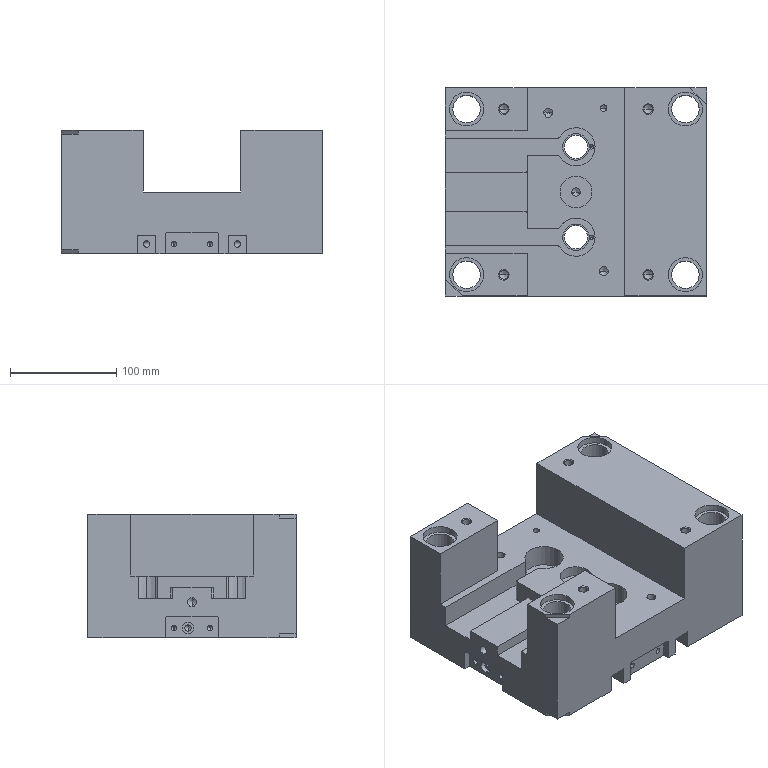Part | STEP file | 2 | 1 solid | 243 faces | box 246 x 196 x 116 mm | volume 3430597 mm3 | cylinder 118 | plane 63 | cone 62 | commonest cylinder face diameters 5 x20 6 x20 4 x16 8.5 x14 8.376 x8 26 x8